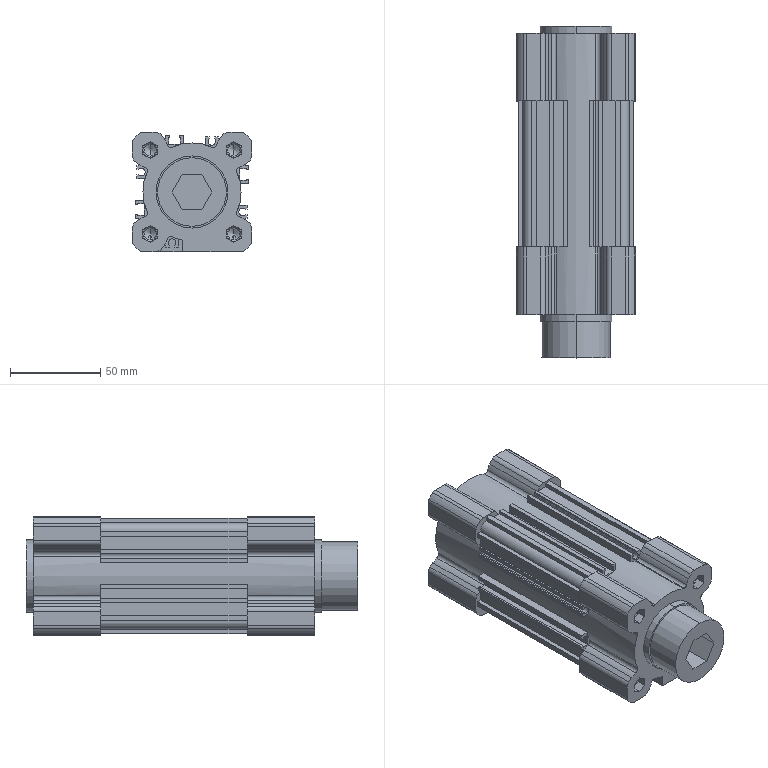Part | SolidWorks | features BaseBody 1 | 1 solid | 425 faces | box 66 x 184 x 66 mm | volume 425451 mm3 | plane 265 | cylinder 120 | cone 40 | commonest cylinder face diameters 7 x30 4 x17 6.647 x16 20 x14 4.25 x9 22 x8